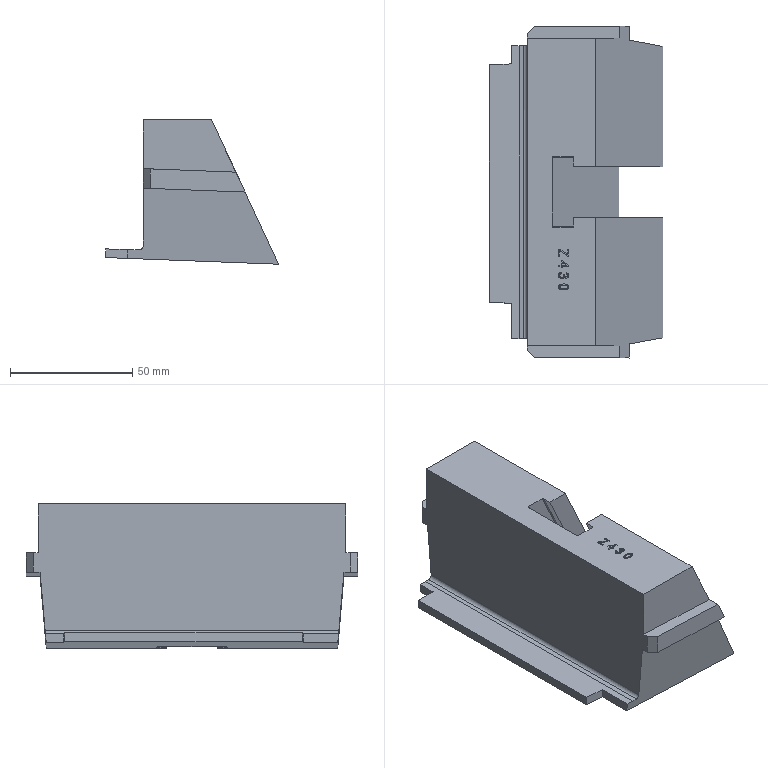Part | Creo | 1 solid | 118 faces | box 71.106 x 136 x 59.157 mm | volume 281390 mm3 | plane 57 | other 55 | cylinder 6 | commonest cylinder face diameters 1 x4 3 x1 57.356 x1